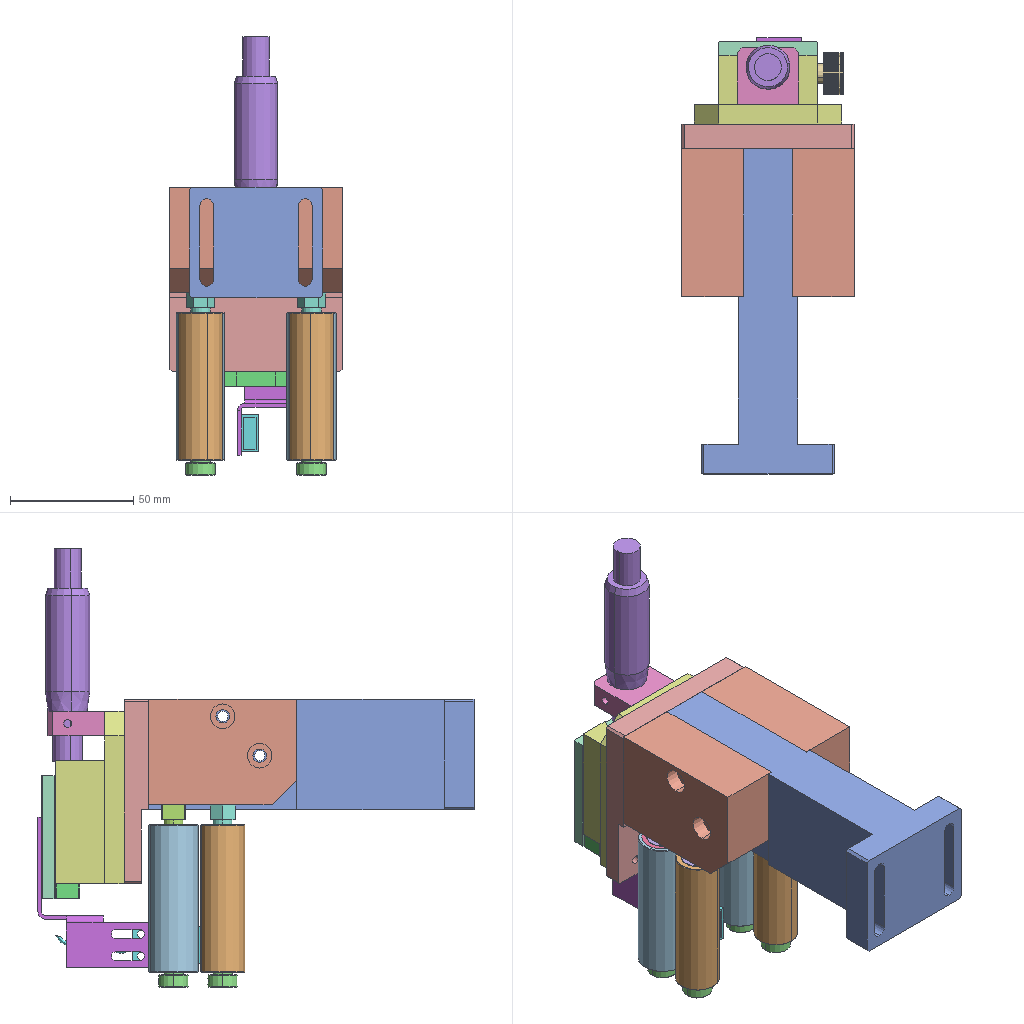Assembly | SolidWorks | 20 different items | 39 placed | box 70 x 177 x 178 mm
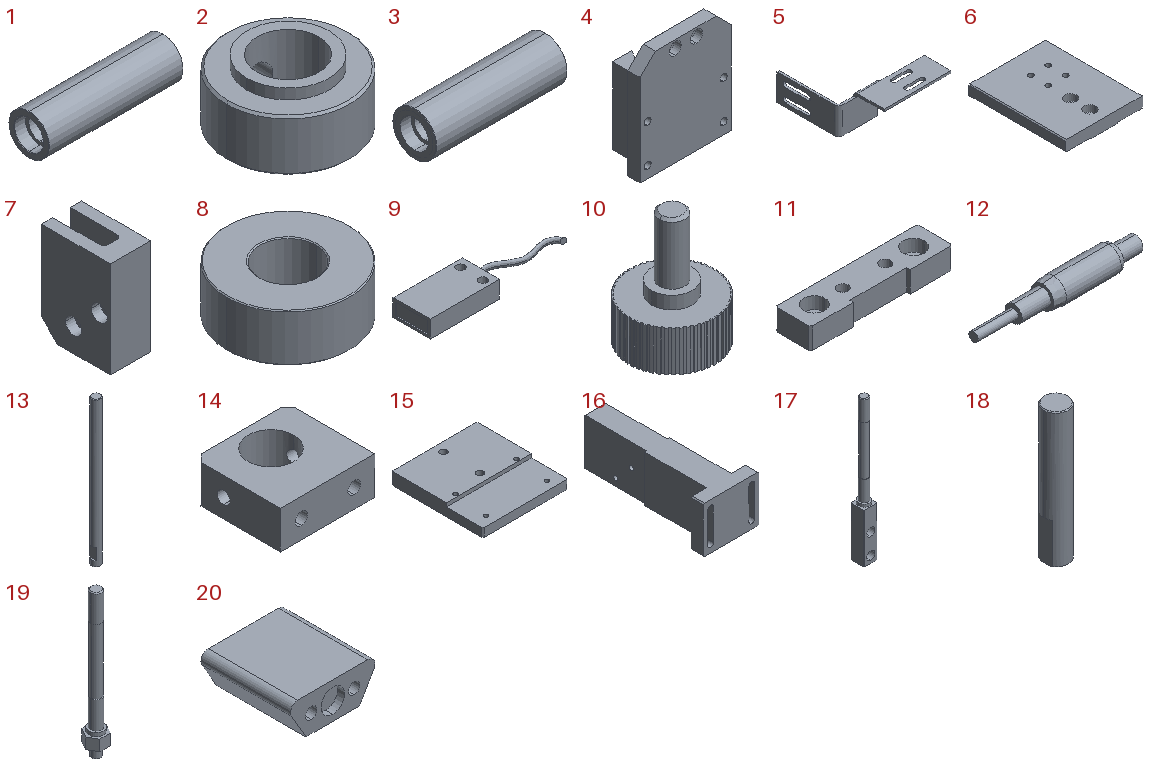Parts list (item | quantity | size | volume | features):
1 | x2 | 60 x 18 x 18 mm | 10010 mm3 | features Chamfer 1, Revolution 1
2 | x4 | 12 x 12 x 6 mm | 429.723 mm3 | features ICE 2, Chamfer 1, Extrusion 1, HoleWzd 1
3 | x2 | 60 x 20 x 20 mm | 13593 mm3 | features Chamfer 1, ICE 1, Revolution 1
4 | x1 | 60 x 28 x 70 mm | 60781 mm3 | features HoleWzd 4, ICE 2, Chamfer 1, Extrusion 1
5 | x1 | 56.5 x 61 x 21 mm | 2744 mm3 | features ICE 4, Fillet 2, ExtruThin 1
6 | x1 | 40 x 50 x 6 mm | 10973 mm3 | features HoleWzd 2, Chamfer 1, Extrusion 1
7 | x2 | 25 x 43 x 60 mm | 52807 mm3 | features ICE 9, HoleWzd 3, Chamfer 1, Cut 1, ExtruThin 1, Fillet 1
8 | x8 | 13 x 13 x 5 mm | 521.693 mm3 | features Chamfer 1, Extrusion 1
9 | x1 | 59.032 x 15 x 7 mm | 2869 mm3 | features Extrusion 1, ICE 1, Sweep 1
10 | x1 | 16.993 x 17 x 22.5 mm | 2126 mm3 | features ICE 3, Chamfer 1, CirPattern 1, Extrusion 1
11 | x1 | 40 x 10 x 6 mm | 1941 mm3 | features HoleWzd 2, Chamfer 1, Cut 1, Extrusion 1, ICE 1
12 | x1 | 115 x 18 x 18 mm | 17209 mm3 | features Revolution 1
13 | x2 | 3 x 3 x 50 mm | 349.971 mm3 | features Chamfer 1, Extrusion 1, ICE 1
14 | x1 | 25 x 23 x 10 mm | 4270 mm3 | features HoleWzd 2, Chamfer 1, Extrusion 1, ICE 1, MirrorPattern 1
15 | x1 | 70 x 75 x 10 mm | 44793 mm3 | features HoleWzd 2, Chamfer 1, Extrusion 1, ICE 1
16 | x1 | 54 x 132 x 45 mm | 142452 mm3 | features HoleWzd 3, ICE 2, Chamfer 1, Extrusion 1
17 | x2 | 10 x 10 x 104 mm | 4818 mm3 | features ICE 3, Chamfer 2, Extrusion 1, RefAxis 1, RevCut 1
18 | x4 | 6 x 6 x 33 mm | 921.126 mm3 | features Chamfer 1, Extrusion 1, ICE 1
19 | x2 | 11.547 x 10 x 80 mm | 2437 mm3 | features ICE 3, Chamfer 2, Extrusion 1, RefAxis 1, RevCut 1
20 | x1 | 23.619 x 25 x 10 mm | 4394 mm3 | features HoleWzd 2, ICE 2, Extrusion 1
Mates (type | each side: item.copy, entity, surface, feature):
Coincident | 16.1 face plane Boss-Extrude1 | 15.1 face plane Boss-Extrude1 | 2 times
Concentric | 17.1 face cylinder Boss-Extrude3 | 3.1 face cylinder Revolve1
Coincident | 17.1 face plane Boss-Extrude2 | 8.1 face plane Boss-Extrude1
Coincident | 17.1 face plane Boss-Extrude3 | 2.1 face plane Boss-Extrude1
Concentric | 17.1 face cylinder Boss-Extrude3 | 2.1 face cylinder Cut-Extrude1
Concentric | 19.1 face cylinder Boss-Extrude4 | 1.1 face cylinder Revolve1
Coincident | 19.1 face plane Boss-Extrude3 | 8.2 face plane Boss-Extrude1
Concentric | 19.1 face cylinder Boss-Extrude4 | 2.2 face cylinder Boss-Extrude1
Concentric | 1.1 face cylinder Revolve1 | 8.2 face cylinder Boss-Extrude1
Coincident | 1.1 face plane Revolve1 | 8.2 face plane Boss-Extrude1
Concentric | 1.1 face cylinder Revolve1 | 8.3 face cylinder Boss-Extrude1
Coincident | 1.1 face plane Revolve1 | 8.3 face plane Boss-Extrude1
Coincident | 8.3 face plane Boss-Extrude1 | 2.2 face plane Boss-Extrude2
Concentric | 3.1 face cylinder Revolve1 | 8.1 face cylinder Boss-Extrude1
Coincident | 3.1 face plane Revolve1 | 8.1 face plane Boss-Extrude1
Concentric | 3.1 face cylinder Revolve1 | 8.4 face cylinder Boss-Extrude1
Coincident | 3.1 face plane Revolve1 | 8.4 face plane Boss-Extrude1
Concentric | 17.2 face cylinder Boss-Extrude3 | 3.2 face cylinder Revolve1
Coincident | 17.2 face plane Boss-Extrude2 | 8.5 face plane Boss-Extrude1
Coincident | 17.2 face plane Boss-Extrude3 | 2.3 face plane Boss-Extrude1
Concentric | 17.2 face cylinder Boss-Extrude3 | 2.3 face cylinder Cut-Extrude1
Concentric | 19.2 face cylinder Boss-Extrude4 | 1.2 face cylinder Revolve1
Coincident | 19.2 face plane Boss-Extrude3 | 8.6 face plane Boss-Extrude1
Concentric | 19.2 face cylinder Boss-Extrude4 | 2.4 face cylinder Boss-Extrude1
Concentric | 1.2 face cylinder Revolve1 | 8.6 face cylinder Boss-Extrude1
Coincident | 1.2 face plane Revolve1 | 8.6 face plane Boss-Extrude1
Concentric | 1.2 face cylinder Revolve1 | 8.7 face cylinder Boss-Extrude1
Coincident | 1.2 face plane Revolve1 | 8.7 face plane Boss-Extrude1
Coincident | 8.7 face plane Boss-Extrude1 | 2.4 face plane Boss-Extrude2
Concentric | 3.2 face cylinder Revolve1 | 8.5 face cylinder Boss-Extrude1
Coincident | 3.2 face plane Revolve1 | 8.5 face plane Boss-Extrude1
Concentric | 3.2 face cylinder Revolve1 | 8.8 face cylinder Boss-Extrude1
Coincident | 3.2 face plane Revolve1 | 8.8 face plane Boss-Extrude1
Coincident | 6.1 face plane Boss-Extrude1 | 5.1 face plane Extrude-Thin1
Width | 5.1 face plane Cut-Extrude3 | 5.1 face plane Cut-Extrude3 | 6.1 face cylinder M3 Tapped Hole1
Coincident | 4.1 face plane Boss-Extrude1 | 15.1 face plane Boss-Extrude1
Concentric | 16.1 face cylinder M5 Tapped Hole2 | 7.1 face cylinder Hole Size per Socket Head Cap Screw Type1 | 2 times
Coincident | 18.1 face cylinder Boss-Extrude1 | 7.1 edge
Coincident | 18.1 face plane Boss-Extrude1 | 7.1 face plane Cut-Extrude3
Concentric | 18.2 face cylinder Boss-Extrude1 | 7.1 face cylinder Cut-Extrude3
Coincident | 18.2 face plane Boss-Extrude1 | 18.1 face plane Boss-Extrude1
Concentric | 17.1 face cylinder Cut-Extrude1 | 18.2 face cylinder Boss-Extrude1
Concentric | 17.1 face cylinder Cut-Extrude1 | 18.1 face cylinder Boss-Extrude1
DistanceDim | 17.1 face plane Boss-Extrude1 | 7.1 face plane Cut-Extrude2
Concentric | 19.1 face cylinder Boss-Extrude2 | 7.1 face cylinder M5 Tapped Hole1
Coincident | 19.1 face plane Boss-Extrude1 | 7.1 face plane Extrude-Thin1
Coincident | 16.1 face plane Cut-Extrude1 | 7.1 face plane Extrude-Thin1
Concentric | 16.1 face cylinder M5 Tapped Hole2 | 7.2 face cylinder Hole Size per Socket Head Cap Screw Type1 | 2 times
Concentric | 18.3 face cylinder Boss-Extrude1 | 7.2 face cylinder Cut-Extrude3
Coincident | 18.3 face plane Boss-Extrude1 | 7.2 face plane Cut-Extrude3
Concentric | 18.4 face cylinder Boss-Extrude1 | 7.2 face cylinder Cut-Extrude3
Coincident | 18.4 face plane Boss-Extrude1 | 18.3 face plane Boss-Extrude1
Concentric | 17.2 face cylinder Cut-Extrude1 | 18.3 face cylinder Boss-Extrude1
Concentric | 17.2 face cylinder Cut-Extrude1 | 18.4 face cylinder Boss-Extrude1
DistanceDim | 17.2 face plane Boss-Extrude1 | 7.2 face plane Cut-Extrude2
Coincident | 19.2 face plane Boss-Extrude1 | 7.2 face plane Extrude-Thin1
Concentric | 19.2 face cylinder Boss-Extrude2 | 7.2 face cylinder M5 Tapped Hole1
Coincident | 16.1 face plane Cut-Extrude1 | 7.2 face plane Extrude-Thin1
Coincident | 15.1 face plane Boss-Extrude1 | 7.2 face plane Extrude-Thin1
Width | 15.1 face plane Boss-Extrude1 | 15.1 face plane Boss-Extrude1 | 4.1 face plane Boss-Extrude2 | 4.1 face plane Boss-Extrude2
Coincident | 15.1 face plane Boss-Extrude1 | 4.1 face plane Boss-Extrude2
Concentric | 4.1 face cylinder Hole Size per Socket Head Cap Screw Type1 | 14.1 edge
Concentric | 4.1 face cylinder Hole Size per Socket Head Cap Screw Type1 | 14.1 face cylinder M4 Tapped Hole1
Coincident | 4.1 face plane Boss-Extrude2 | 14.1 face plane Boss-Extrude1
Concentric | 20.1 face cylinder Cut-Extrude1 | 13.1 face cylinder Boss-Extrude1
Concentric | 20.1 face cylinder Cut-Extrude1 | 13.2 face cylinder Boss-Extrude1
Coincident | 13.1 face plane Boss-Extrude1 | 13.2 face plane Boss-Extrude1
Coincident | 4.1 face plane Cut-Extrude1 | 20.1 face plane Boss-Extrude1
Width | 20.1 face plane Boss-Extrude1 | 20.1 face plane Boss-Extrude1 | 4.1 face plane Cut-Extrude1 | 4.1 face plane Cut-Extrude1
Concentric | 6.1 face cylinder Hole Size per Socket Head Cap Screw Type1 | 20.1 face cylinder M3 Tapped Hole1 | 2 times
Coincident | 6.1 face plane Boss-Extrude1 | 20.1 face plane Boss-Extrude1
Parallel | 5.1 face plane Extrude-Thin1 | 6.1 face plane Boss-Extrude1
Coincident | 4.1 face plane Boss-Extrude1 | 11.1 face plane Boss-Extrude1
Concentric | 4.1 face cylinder M3 Tapped Hole1 | 11.1 face cylinder Hole Size per Socket Head Cap Screw Type1 | 2 times
Coincident | 4.1 face plane Boss-Extrude1 | 10.1 face plane Boss-Extrude2
Concentric | 4.1 face cylinder M5 Tapped Hole1 | 10.1 face cylinder Boss-Extrude3
Concentric | 14.1 face cylinder Cut-Extrude1 | 12.1 face cylinder Revolve1
Coincident | 14.1 face plane Boss-Extrude1 | 12.1 face plane Revolve1
Coincident | 5.1 face plane Boss-Extrude1 | 9.1 face plane Boss-Extrude1
Width | 5.1 face plane Boss-Extrude1 | 5.1 face plane Cut-Extrude2 | 9.1 face plane Boss-Extrude1 | 9.1 face plane Boss-Extrude1
Coincident | 13.2 face plane Boss-Extrude1 | 11.1 face plane Boss-Extrude1